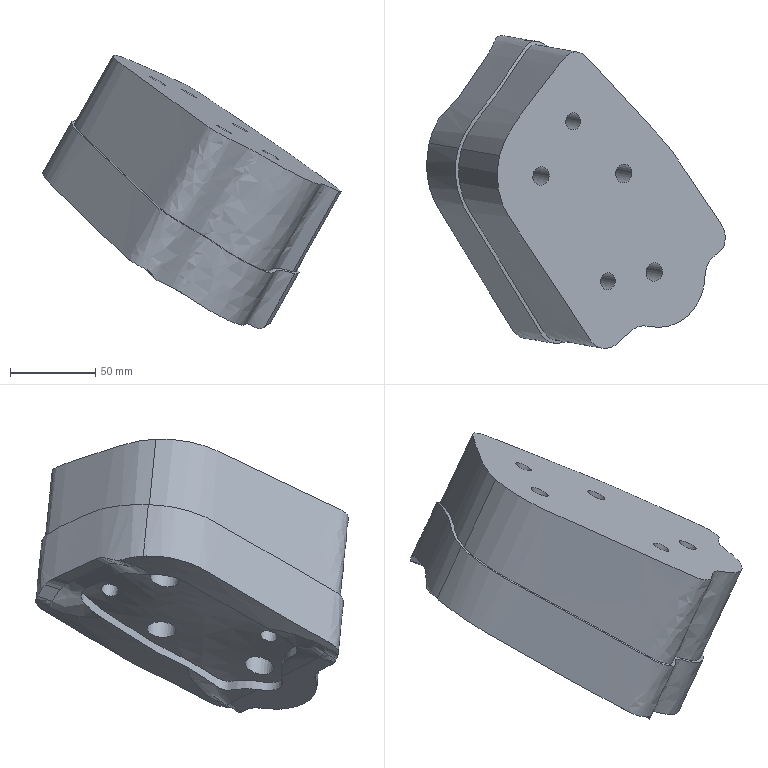Part | NX | features solid 2 | 1 solid | 50 faces | box 175.408 x 183.768 x 160.813 mm | volume 1317946 mm3 | spline 38 | cylinder 8 | plane 4 | commonest cylinder face diameters 11 x3 17 x3 10 x2